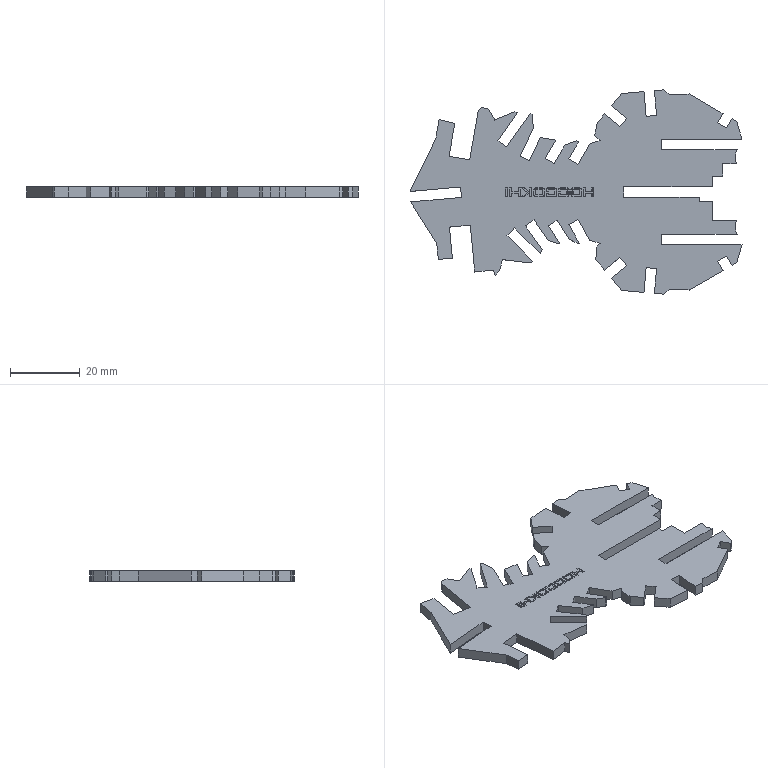Part | SolidWorks | features BaseBody 1 | 1 solid | 229 faces | box 94.912 x 58.414 x 3 mm | volume 9467 mm3 | plane 213 | spline 16